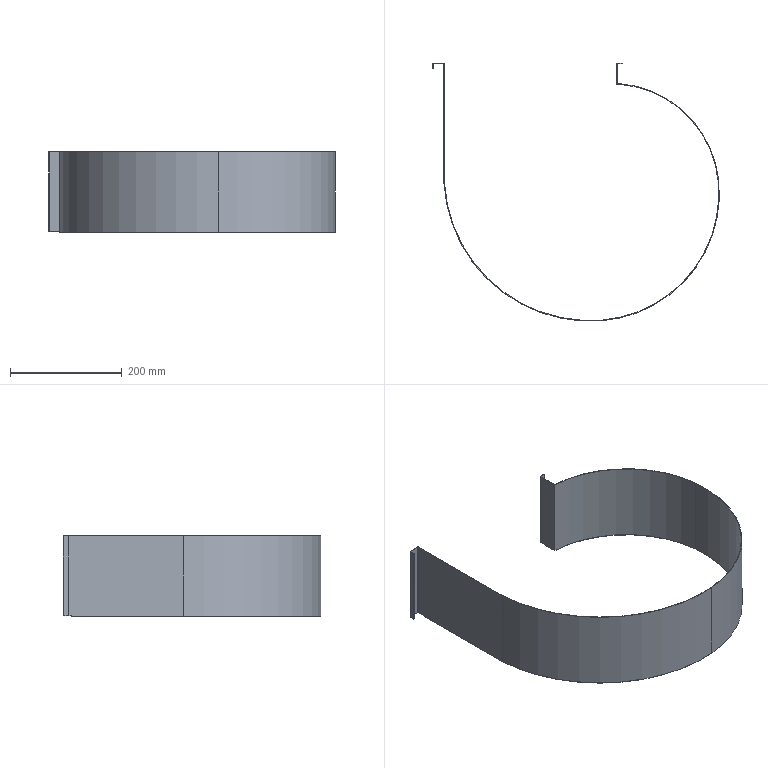Part | STEP file | HESS-408-70-15W-N-8-inner liner turbine enclosure plate | 1 solid | 34 faces | box 512.743 x 461.634 x 144 mm | volume 193062 mm3 | plane 18 | cylinder 16 | commonest cylinder face diameters 0.2 x5 2.2 x5 385.951 x1 387.951 x1 454.243 x1 456.243 x1